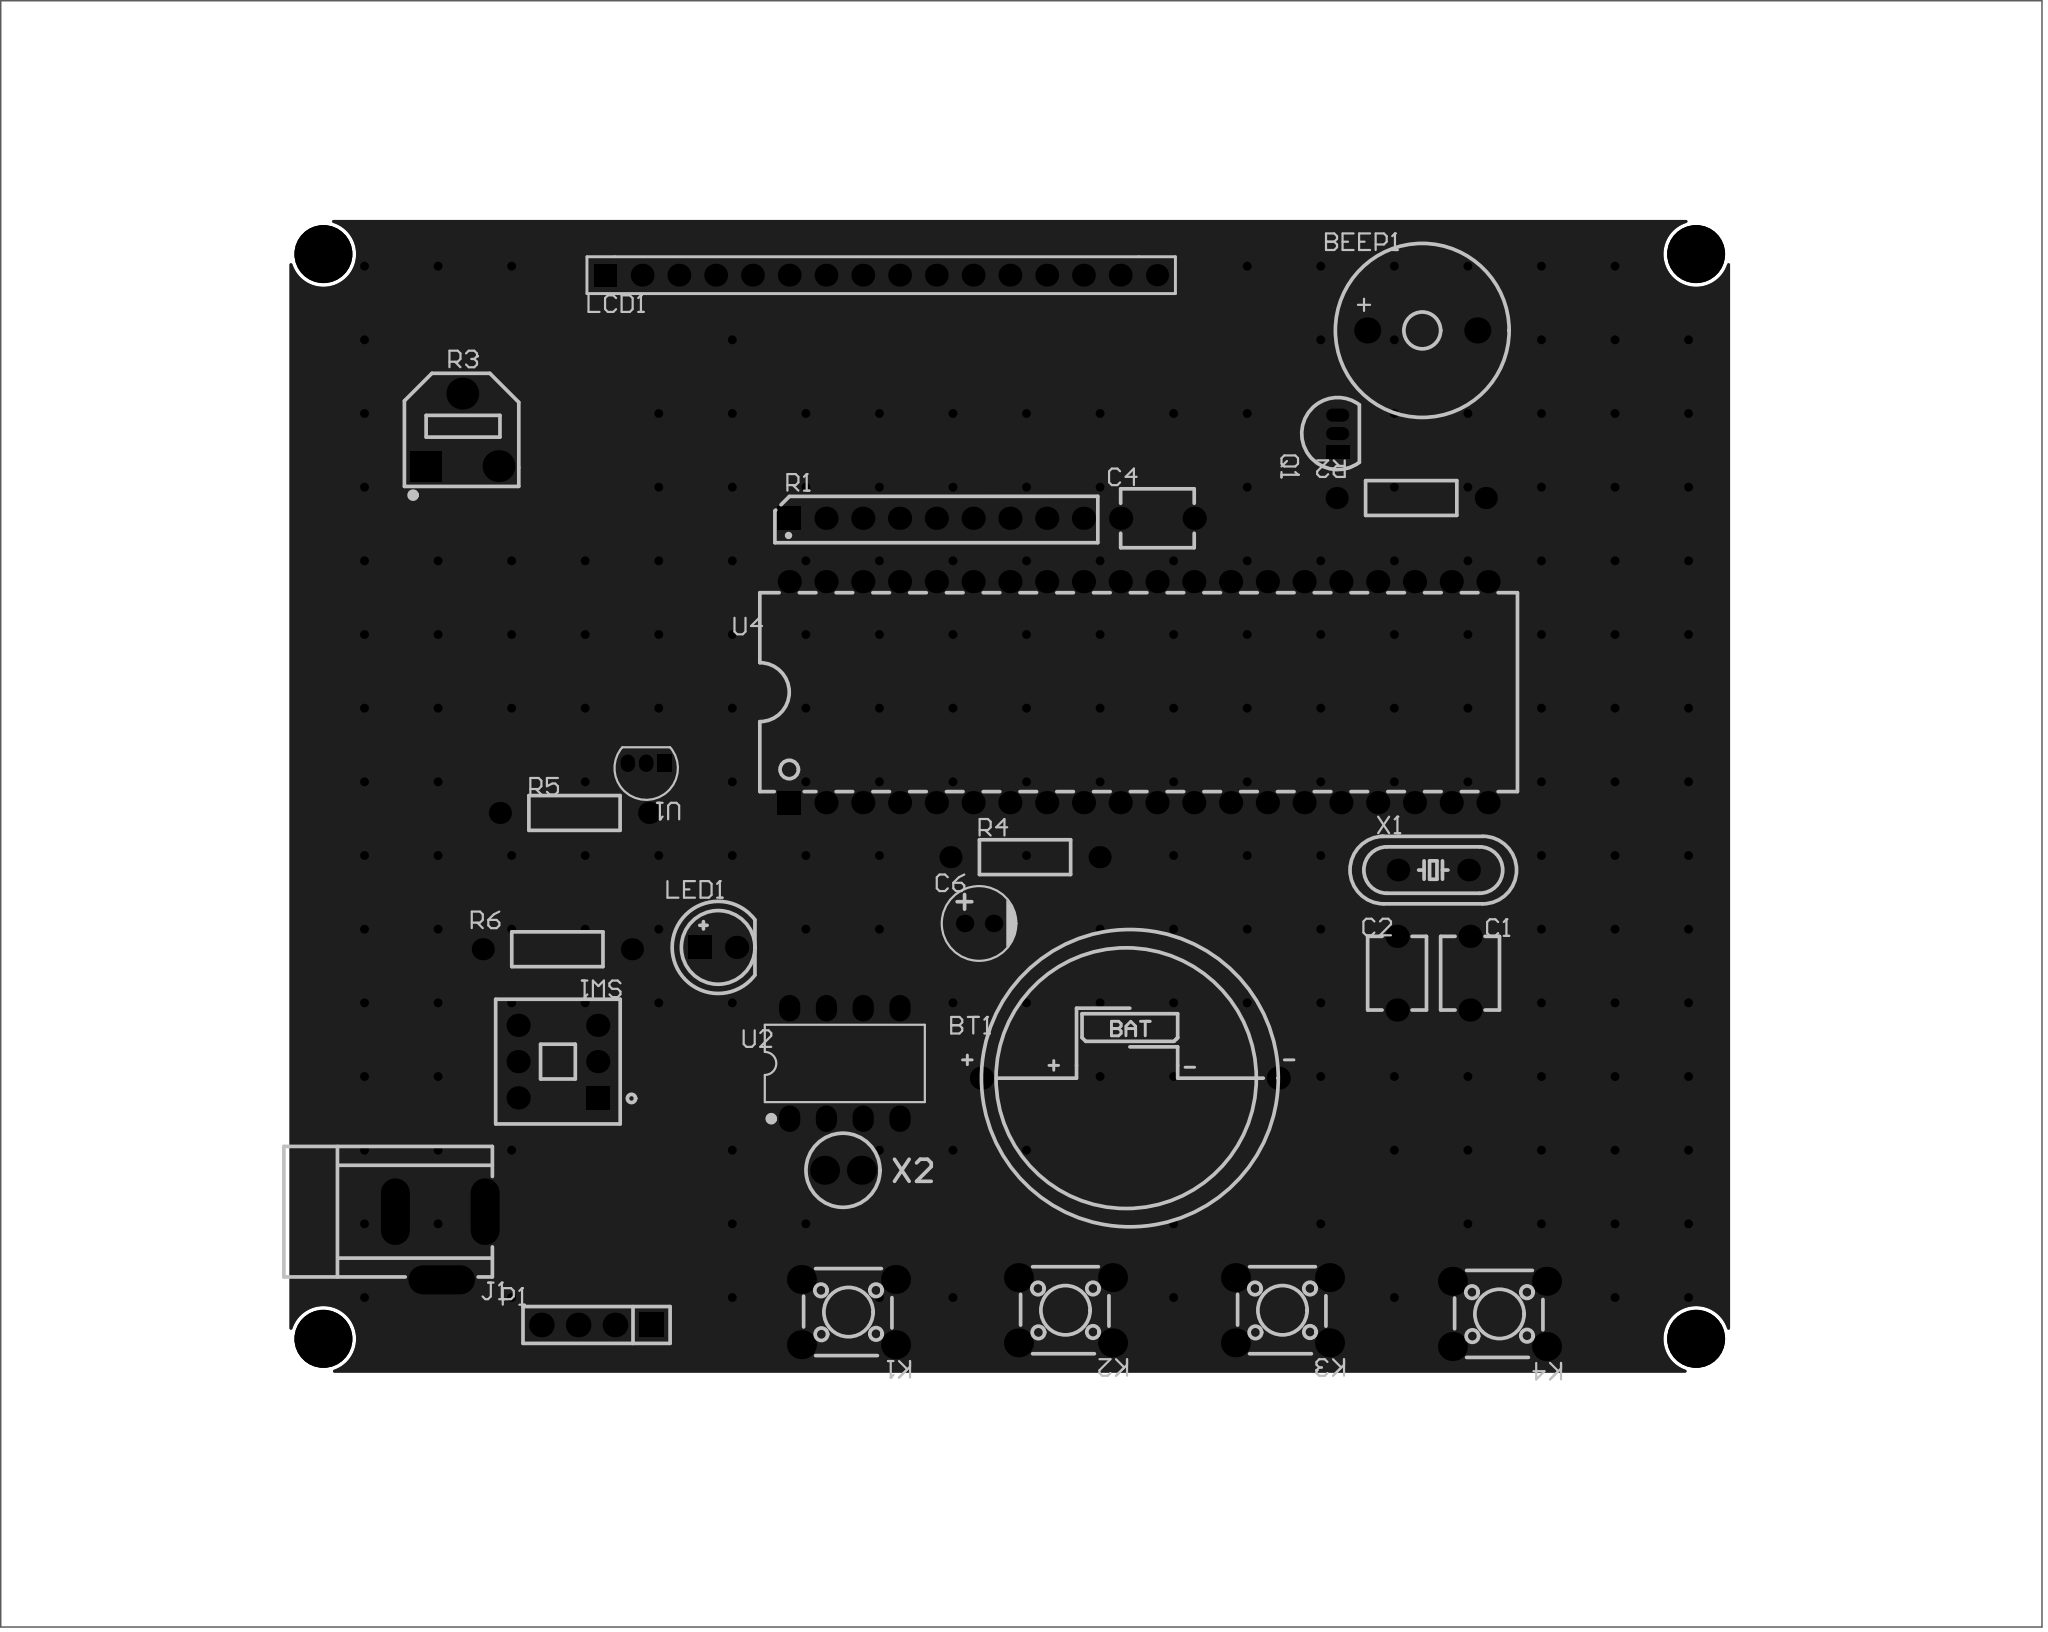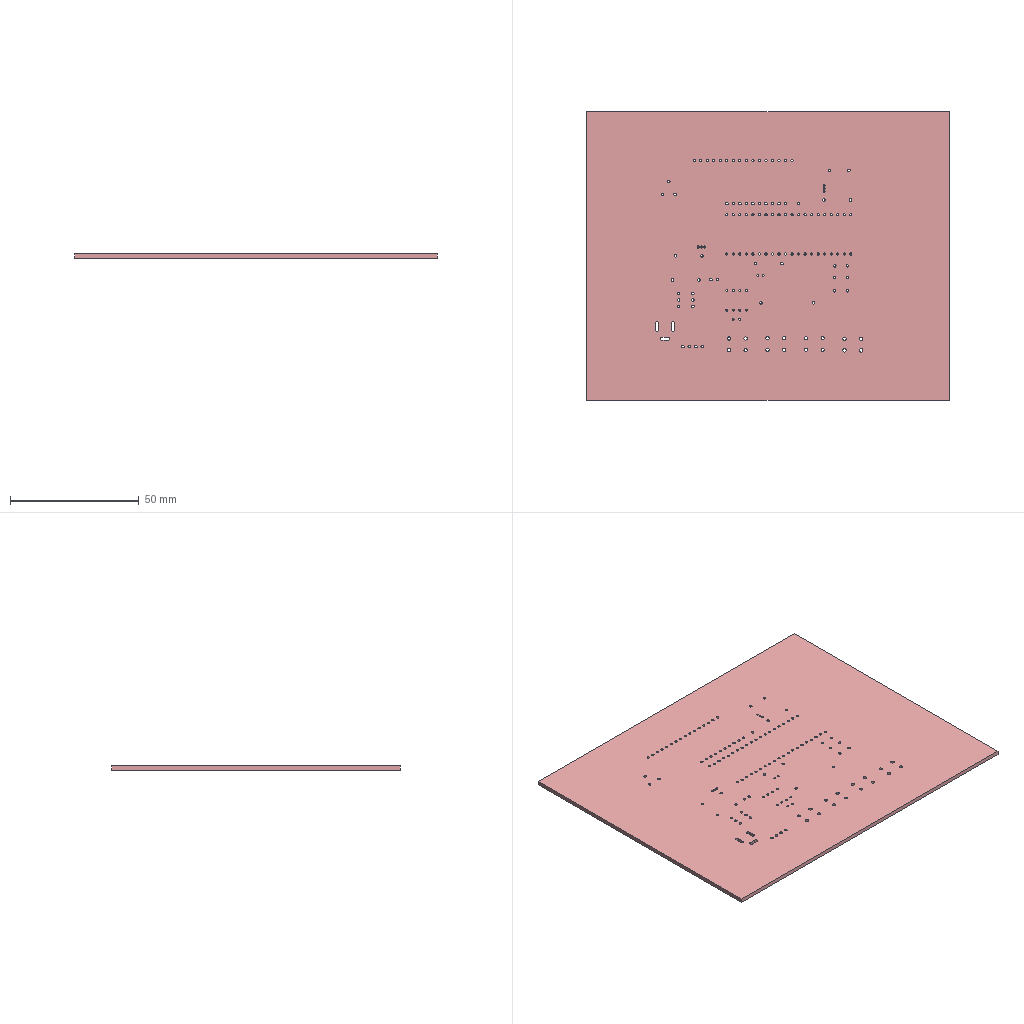Circuit board layout | Altium Designer | box 141 x 112.1 x 1.6 mm
Layer stack:
# Altium Designer layer stack of  (unit mm; dielectric type: 0 none, 1 core, 2 prepreg, 3 surface material)
index,name,kind,layer,copper_thickness_mm,dielectric_type,dielectric_thickness_mm,dielectric_material,dielectric_constant
0,Top Paste Mask Layer,other,,,,,,
1,Top Silkscreen Layer,other,,,,,,
2,Top Solder Mask Layer,dielectric,,,3,0.01,,3.3
3,Top Layer,copper,Top Layer,0.035,,,,
4,Dielectric1,dielectric,,,3,1.51,FR4,4.5
5,Bottom Layer,copper,Bottom Layer,0.035,,,,
6,Bottom Solder Mask Layer,dielectric,,,3,0.01,,3.3
7,Bottom Silkscreen Layer,other,,,,,,
8,Bottom Paste Mask Layer,other,,,,,,
# drill layer pairs: low layer,high layer
drill_pair,Top Layer,Bottom Layer
Part placement:
Designator,Comment,Layer,Footprint,Center-X(mm),Center-Y(mm),Rotation
BEEP1,,TopLayer,BUZ-TH_BD12.0-P7.60-D0.6-FD,168.021,159.258,0
BT1,Battery,TopLayer,BAT-TH_CR2032,147.828,107.696,0
C6,10uF,TopLayer,CAP-TH_BD5.0-P2.00-D0.6-FD,137.414,118.364,0
J1,,TopLayer,DC-005_2.5,100.203,96.139,180
LCD1,1602,TopLayer,HDR-M-2.54_1X16,130.655,163.068,0
Q1,8550,TopLayer,S8550P_TO-92,162.179,152.146,90
SW1,SWT,TopLayer,SW-TH_6P-L8.5-W8.5-P2.50-LS5.5-BL-2,108.331,108.839,90
U1,DS18B20,TopLayer,TO-92-3_L4.5-W3.5-P1.27-L,114.427,129.413,180
U2,DS1302,TopLayer,DIP-8_L10.9-W6.4-P2.54-LS7.6-BL,128.143,108.712,0
U4,STC89C52RC-40I-PDIP40,TopLayer,DIP-40_L52.0-W13.7-P2.54-LS15.2-BL,148.435,134.314,0
X1,12M,TopLayer,HC-49S_L11.5-W4.7-P4.88,168.783,122.047,0
R1,,TopLayer,SIP-9_L22.3-W3.2-P2.54_KA2284-SIP-9,134.465,146.304,0
LED1,,TopLayer,LED-TH_5mm,119.396,116.713,0
P1,,TopLayer,HDR-TH_4P-P2.54-V-M,110.998,90.678,180
R2,1K,TopLayer,Res_1/4W,167.259,147.701,0
R4,10K,TopLayer,Res_1/4W,140.589,122.936,0
R5,4.7K,TopLayer,Res_1/4W,109.474,125.984,180
R6,1K,TopLayer,Res_1/4W,108.291,116.586,0
R3,103,TopLayer,RES-ADJ-SMD_RM065-V1,101.727,152.4,0
K1,,TopLayer,KEY-TH_4P-L6.0-W6.0-P4.50-LS6.50,128.397,91.567,180
K2,,TopLayer,KEY-TH_4P-L6.0-W6.0-P4.50-LS6.50,143.383,91.694,180
K3,,TopLayer,KEY-TH_4P-L6.0-W6.0-P4.50-LS6.50,158.369,91.694,180
K4,,TopLayer,KEY-TH_4P-L6.0-W6.0-P4.50-LS6.50,173.355,91.44,180
C4,0.1uF,TopLayer,CAP-TH_L5.0-W4.0-P5.00-D1.0,149.733,146.304,0
C1,30pF,TopLayer,CAP-TH_L5.0-W4.0-P5.00-D1.0,171.323,114.935,90
C2,30pF,TopLayer,CAP-TH_L5.0-W4.0-P5.00-D1.0,166.281,114.935,90
X2,32.768kHz,TopLayer,XTAL2,128.016,101.346,180
Pad and via stacks:
# Altium Designer via and pad stacks of  (unit mm). Each distinct definition once, with the count of objects using it.
# via: kind,start_layer,end_layer,hole_mm,diameter_mm,mode(0 simple;1 top-mid-bottom;2 full stack),diameter_per_layer,count,example_net
# pad: kind,layer,hole_mm,hole_type(0 round;1 square;2 slot),plating,top_size,top_shape(1 round;2 rect;3 octagon;9 rounded rect),mid_size,bottom_size,mode,footprint,size_per_layer,count,example
pad,Multi-Layer,1,0,plated,1.8x1.8,1,1.8x1.8,1.8x1.8,0,BUZ-TH_BD12.0-P7.60-D0.6-FD,,2,BEEP1.2
pad,Multi-Layer,1,0,plated,1.6x1.6,1,1.6x1.6,1.6x1.6,0,BAT-TH_CR2032,,2,BT1.1
pad,Multi-Layer,0.801,0,plated,1.202x1.202,1,1.202x1.202,1.202x1.202,0,CAP-TH_BD5.0-P2.00-D0.6-FD,,2,C6.1
pad,Multi-Layer,1.2,2,plated,2x4.6,1,2x4.6,2x4.6,0,DC-005_2.5,,2,J1.1
pad,Multi-Layer,1.2,2,plated,4.6x2,1,4.6x2,4.6x2,0,DC-005_2.5,,1,J1.3
pad,Multi-Layer,0.889,0,plated,1.575x1.575,1,1.575x1.575,1.575x1.575,0,HDR-M-2.54_1X16,,14,LCD1.15
pad,Multi-Layer,0.889,0,plated,1.575x1.575,2,1.575x1.575,1.575x1.575,0,HDR-M-2.54_1X16,,1,LCD1.1
pad,Multi-Layer,0.9144,0,plated,1.524x1.524,1,1.524x1.524,1.524x1.524,0,HDR-M-2.54_1X16,,1,LCD1.16
pad,Multi-Layer,0.7,0,plated,0.9x1.6,1,0.9x1.6,0.9x1.6,0,S8550P_TO-92,,2,Q1.3
pad,Multi-Layer,0.7,0,plated,0.9x1.6,2,0.9x1.6,0.9x1.6,0,S8550P_TO-92,,1,Q1.1
pad,Multi-Layer,1,0,plated,1.6x1.6,2,1.6x1.6,1.6x1.6,0,SW-TH_6P-L8.5-W8.5-P2.50-LS5.5-BL-2,,1,SW1.1
pad,Multi-Layer,1,0,plated,1.6x1.6,1,1.6x1.6,1.6x1.6,0,SW-TH_6P-L8.5-W8.5-P2.50-LS5.5-BL-2,,5,SW1.2
pad,Multi-Layer,0.7,2,plated,1x1.2,2,1x1.2,1x1.2,0,TO-92-3_L4.5-W3.5-P1.27-L,,1,U1.1
pad,Multi-Layer,0.7,2,plated,1x1.2,1,1x1.2,1x1.2,0,TO-92-3_L4.5-W3.5-P1.27-L,,2,U1.2
pad,Multi-Layer,0.8,0,plated,1.462x1.827,1,1.462x1.827,1.462x1.827,0,DIP-8_L10.9-W6.4-P2.54-LS7.6-BL,,8,U2.1
pad,Multi-Layer,0.889,0,plated,1.6x1.6,1,1.6x1.6,1.6x1.6,0,DIP-40_L52.0-W13.7-P2.54-LS15.2-BL,,39,U4.31
pad,Multi-Layer,0.889,0,plated,1.6x1.6,2,1.6x1.6,1.6x1.6,0,DIP-40_L52.0-W13.7-P2.54-LS15.2-BL,,1,U4.1
pad,Multi-Layer,0.9,0,plated,1.56x1.56,1,1.56x1.56,1.56x1.56,0,HC-49S_L11.5-W4.7-P4.88,,2,X1.2
pad,Multi-Layer,1,0,plated,1.6x1.6,2,1.6x1.6,1.6x1.6,0,SIP-9_L22.3-W3.2-P2.54_KA2284-SIP-9,,1,R1.1
pad,Multi-Layer,1,0,plated,1.6x1.6,1,1.6x1.6,1.6x1.6,0,SIP-9_L22.3-W3.2-P2.54_KA2284-SIP-9,,8,R1.2
pad,Multi-Layer,1,0,plated,1.6x1.6,2,1.6x1.6,1.6x1.6,0,LED-TH_5mm,,1,LED1.1
pad,Multi-Layer,1,0,plated,1.6x1.6,1,1.6x1.6,1.6x1.6,0,LED-TH_5mm,,1,LED1.2
pad,Multi-Layer,1.1,0,plated,1.7x1.7,2,1.7x1.7,1.7x1.7,0,HDR-TH_4P-P2.54-V-M,,1,P1.1
pad,Multi-Layer,1.1,0,plated,1.7x1.7,1,1.7x1.7,1.7x1.7,0,HDR-TH_4P-P2.54-V-M,,3,P1.2
pad,Multi-Layer,1,0,plated,1.524x1.524,1,1.524x1.524,1.524x1.524,0,Res_1/4W,,8,R2.1
pad,Multi-Layer,1,0,plated,2.2x2.1,2,2.2x2.1,2.2x2.1,0,RES-ADJ-SMD_RM065-V1,,1,R3.1
pad,Multi-Layer,1,0,plated,2.2x2.2,1,2.2x2.2,2.2x2.2,0,RES-ADJ-SMD_RM065-V1,,2,R3.3
pad,Multi-Layer,1.3,0,plated,2x2,1,2x2,2x2,0,KEY-TH_4P-L6.0-W6.0-P4.50-LS6.50,,16,K1.4
pad,Multi-Layer,1,0,plated,1.6x1.6,1,1.6x1.6,1.6x1.6,0,CAP-TH_L5.0-W4.0-P5.00-D1.0,,6,C4.1
pad,Multi-Layer,0.762,0,plated,2x2,1,2x2,2x2,0,XTAL2,,2,X2.1
via,Top Layer,Bottom Layer,3,4,0,,4,
via,Top Layer,Bottom Layer,0.3048,0.61,0,,204,GND
Copper pours:
name,layer,net,type(0 solid;1 hatched;2 none)
Bottom Layer-GND,Bottom Layer,GND,0
Top Layer-GND,Top Layer,GND,0